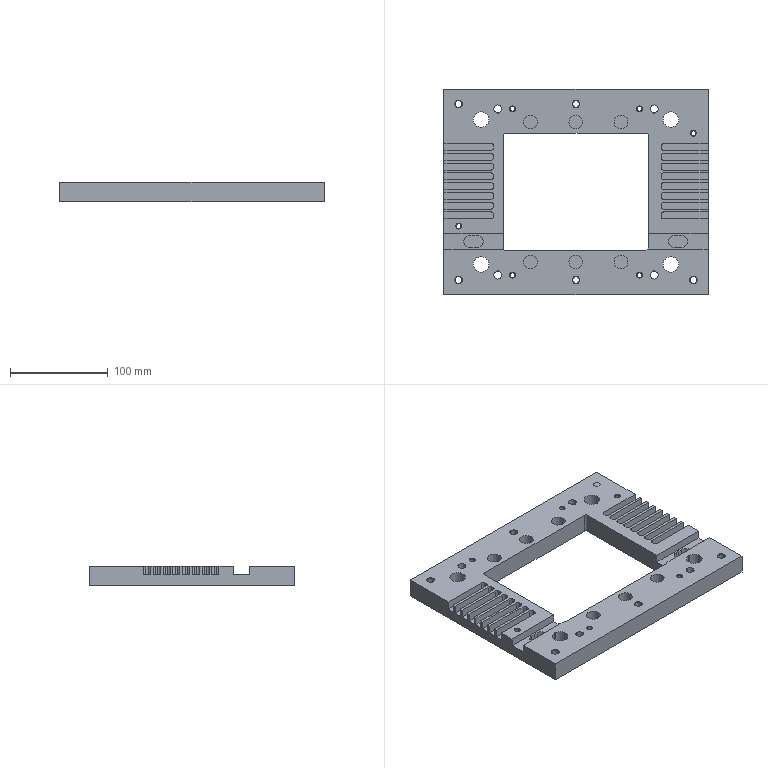Part | STEP file | 1 solid | 220 faces | box 270 x 210 x 20 mm | volume 665006 mm3 | plane 101 | cylinder 93 | cone 26 | commonest cylinder face diameters 5 x38 1 x24 6.8 x6 14 x6 8.01 x4 11.999 x4